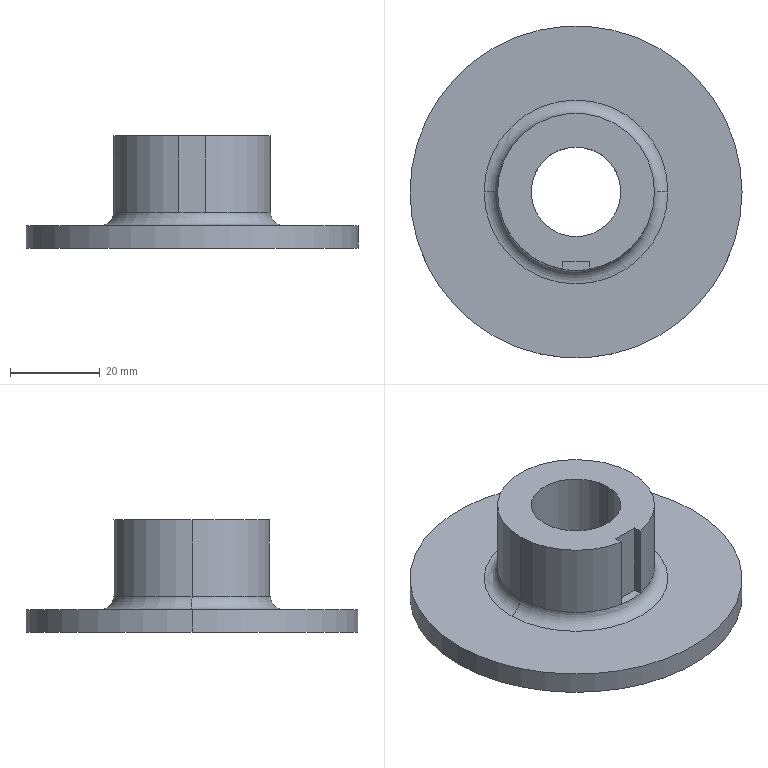Part | SolidWorks | features ICE 3, Extrusion 1, Fillet 1 | 1 solid | 16 faces | box 74 x 74 x 25 mm | volume 32918 mm3 | cylinder 7 | plane 7 | torus 2 | commonest cylinder face diameters 35 x3 20 x2 74 x2
STEP:
#1=CARTESIAN_POINT('',(-17.5,0.,8.));
#2=VERTEX_POINT('',#1);
#3=CARTESIAN_POINT('',(-3.,-17.241,8.));
#4=VERTEX_POINT('',#3);
#5=CARTESIAN_POINT('',(0.,0.,8.));
#6=DIRECTION('',(0.,0.,1.));
#7=DIRECTION('',(1.,0.,0.));
#8=AXIS2_PLACEMENT_3D('',#5,#6,#7);
#9=CIRCLE('',#8,17.5);
#10=EDGE_CURVE('',#2,#4,#9,.T.);
#11=ORIENTED_EDGE('',*,*,#10,.F.);
#12=CARTESIAN_POINT('',(-20.5,0.,5.));
#13=VERTEX_POINT('',#12);
#14=CARTESIAN_POINT('',(-20.5,0.,8.));
#15=DIRECTION('',(0.,1.,0.));
#16=DIRECTION('',(-1.,0.,0.));
#17=AXIS2_PLACEMENT_3D('',#14,#15,#16);
#18=CIRCLE('',#17,3.);
#19=EDGE_CURVE('',#2,#13,#18,.T.);
#20=ORIENTED_EDGE('',*,*,#19,.T.);
#21=CARTESIAN_POINT('',(20.5,0.,5.));
#22=VERTEX_POINT('',#21);
#23=CARTESIAN_POINT('',(0.,0.,5.));
#24=DIRECTION('',(0.,0.,-1.));
#25=DIRECTION('',(1.,0.,0.));
#26=AXIS2_PLACEMENT_3D('',#23,#24,#25);
#27=CIRCLE('',#26,20.5);
#28=EDGE_CURVE('',#22,#13,#27,.T.);
#29=ORIENTED_EDGE('',*,*,#28,.F.);
#30=CARTESIAN_POINT('',(17.5,0.,8.));
#31=VERTEX_POINT('',#30);
#32=CARTESIAN_POINT('',(20.5,0.,8.));
#33=DIRECTION('',(0.,-1.,0.));
#34=DIRECTION('',(0.,0.,-1.));
#35=AXIS2_PLACEMENT_3D('',#32,#33,#34);
#36=CIRCLE('',#35,3.);
#37=EDGE_CURVE('',#31,#22,#36,.T.);
#38=ORIENTED_EDGE('',*,*,#37,.F.);
#39=CARTESIAN_POINT('',(3.,-17.241,8.));
#40=VERTEX_POINT('',#39);
#41=CARTESIAN_POINT('',(0.,0.,8.));
#42=DIRECTION('',(0.,0.,1.));
#43=DIRECTION('',(1.,0.,0.));
#44=AXIS2_PLACEMENT_3D('',#41,#42,#43);
#45=CIRCLE('',#44,17.5);
#46=EDGE_CURVE('',#40,#31,#45,.T.);
#47=ORIENTED_EDGE('',*,*,#46,.F.);
#48=CARTESIAN_POINT('',(0.,0.,8.));
#49=DIRECTION('',(0.,0.,1.));
#50=DIRECTION('',(1.,0.,0.));
#51=AXIS2_PLACEMENT_3D('',#48,#49,#50);
#52=CIRCLE('',#51,17.5);
#53=EDGE_CURVE('',#4,#40,#52,.T.);
#54=ORIENTED_EDGE('',*,*,#53,.F.);
#55=EDGE_LOOP('',(#11,#20,#29,#38,#47,#54));
#56=FACE_OUTER_BOUND('',#55,.T.);
#57=CARTESIAN_POINT('',(0.,0.,8.));
#58=DIRECTION('',(0.,0.,1.));
#59=DIRECTION('',(1.,0.,0.));
#60=AXIS2_PLACEMENT_3D('',#57,#58,#59);
#61=TOROIDAL_SURFACE('',#60,20.5,3.);
#62=ADVANCED_FACE('',(#56),#61,.F.);
#63=CARTESIAN_POINT('',(-10.,0.,25.));
#64=VERTEX_POINT('',#63);
#65=CARTESIAN_POINT('',(10.,0.,25.));
#66=VERTEX_POINT('',#65);
#67=CARTESIAN_POINT('',(0.,0.,25.));
#68=DIRECTION('',(0.,0.,1.));
#69=DIRECTION('',(1.,0.,0.));
#70=AXIS2_PLACEMENT_3D('',#67,#68,#69);
#71=CIRCLE('',#70,10.);
#72=EDGE_CURVE('',#64,#66,#71,.T.);
#73=ORIENTED_EDGE('',*,*,#72,.T.);
#74=CARTESIAN_POINT('',(10.,0.,0.));
#75=VERTEX_POINT('',#74);
#76=CARTESIAN_POINT('',(10.,0.,25.));
#77=DIRECTION('',(0.,0.,-1.));
#78=VECTOR('',#77,1000.);
#79=LINE('',#76,#78);
#80=EDGE_CURVE('',#66,#75,#79,.T.);
#81=ORIENTED_EDGE('',*,*,#80,.T.);
#82=CARTESIAN_POINT('',(-10.,0.,0.));
#83=VERTEX_POINT('',#82);
#84=CARTESIAN_POINT('',(0.,0.,0.));
#85=DIRECTION('',(0.,0.,1.));
#86=DIRECTION('',(1.,0.,0.));
#87=AXIS2_PLACEMENT_3D('',#84,#85,#86);
#88=CIRCLE('',#87,10.);
#89=EDGE_CURVE('',#83,#75,#88,.T.);
#90=ORIENTED_EDGE('',*,*,#89,.F.);
#91=CARTESIAN_POINT('',(-10.,0.,25.));
#92=DIRECTION('',(0.,0.,-1.));
#93=VECTOR('',#92,1000.);
#94=LINE('',#91,#93);
#95=EDGE_CURVE('',#64,#83,#94,.T.);
#96=ORIENTED_EDGE('',*,*,#95,.F.);
#97=EDGE_LOOP('',(#73,#81,#90,#96));
#98=FACE_OUTER_BOUND('',#97,.T.);
#99=CARTESIAN_POINT('',(0.,0.,25.));
#100=DIRECTION('',(0.,0.,-1.));
#101=DIRECTION('',(-1.,0.,0.));
#102=AXIS2_PLACEMENT_3D('',#99,#100,#101);
#103=CYLINDRICAL_SURFACE('',#102,10.);
#104=ADVANCED_FACE('',(#98),#103,.F.);
#105=CARTESIAN_POINT('',(17.5,0.,25.));
#106=VERTEX_POINT('',#105);
#107=CARTESIAN_POINT('',(-17.5,0.,25.));
#108=VERTEX_POINT('',#107);
#109=CARTESIAN_POINT('',(0.,0.,25.));
#110=DIRECTION('',(0.,0.,1.));
#111=DIRECTION('',(1.,0.,0.));
#112=AXIS2_PLACEMENT_3D('',#109,#110,#111);
#113=CIRCLE('',#112,17.5);
#114=EDGE_CURVE('',#106,#108,#113,.T.);
#115=ORIENTED_EDGE('',*,*,#114,.F.);
#116=CARTESIAN_POINT('',(17.5,0.,25.));
#117=DIRECTION('',(0.,0.,-1.));
#118=VECTOR('',#117,1000.);
#119=LINE('',#116,#118);
#120=EDGE_CURVE('',#106,#31,#119,.T.);
#121=ORIENTED_EDGE('',*,*,#120,.T.);
#122=CARTESIAN_POINT('',(0.,0.,8.));
#123=DIRECTION('',(0.,0.,1.));
#124=DIRECTION('',(1.,0.,0.));
#125=AXIS2_PLACEMENT_3D('',#122,#123,#124);
#126=CIRCLE('',#125,17.5);
#127=EDGE_CURVE('',#31,#2,#126,.T.);
#128=ORIENTED_EDGE('',*,*,#127,.T.);
#129=CARTESIAN_POINT('',(-17.5,0.,25.));
#130=DIRECTION('',(0.,0.,-1.));
#131=VECTOR('',#130,1000.);
#132=LINE('',#129,#131);
#133=EDGE_CURVE('',#108,#2,#132,.T.);
#134=ORIENTED_EDGE('',*,*,#133,.F.);
#135=EDGE_LOOP('',(#115,#121,#128,#134));
#136=FACE_OUTER_BOUND('',#135,.T.);
#137=CARTESIAN_POINT('',(0.,0.,25.));
#138=DIRECTION('',(0.,0.,-1.));
#139=DIRECTION('',(-1.,0.,0.));
#140=AXIS2_PLACEMENT_3D('',#137,#138,#139);
#141=CYLINDRICAL_SURFACE('',#140,17.5);
#142=ADVANCED_FACE('',(#136),#141,.T.);
#143=CARTESIAN_POINT('',(-3.,-17.241,25.));
#144=VERTEX_POINT('',#143);
#145=CARTESIAN_POINT('',(0.,0.,25.));
#146=DIRECTION('',(0.,0.,1.));
#147=DIRECTION('',(1.,0.,0.));
#148=AXIS2_PLACEMENT_3D('',#145,#146,#147);
#149=CIRCLE('',#148,17.5);
#150=EDGE_CURVE('',#108,#144,#149,.T.);
#151=ORIENTED_EDGE('',*,*,#150,.F.);
#152=ORIENTED_EDGE('',*,*,#133,.T.);
#153=ORIENTED_EDGE('',*,*,#10,.T.);
#154=CARTESIAN_POINT('',(-3.,-17.241,25.));
#155=DIRECTION('',(0.,0.,1.));
#156=VECTOR('',#155,1000.);
#157=LINE('',#154,#156);
#158=EDGE_CURVE('',#4,#144,#157,.T.);
#159=ORIENTED_EDGE('',*,*,#158,.T.);
#160=EDGE_LOOP('',(#151,#152,#153,#159));
#161=FACE_OUTER_BOUND('',#160,.T.);
#162=CARTESIAN_POINT('',(0.,0.,25.));
#163=DIRECTION('',(0.,0.,-1.));
#164=DIRECTION('',(-1.,0.,0.));
#165=AXIS2_PLACEMENT_3D('',#162,#163,#164);
#166=CYLINDRICAL_SURFACE('',#165,17.5);
#167=ADVANCED_FACE('',(#161),#166,.T.);
#168=CARTESIAN_POINT('',(37.,0.,5.));
#169=VERTEX_POINT('',#168);
#170=CARTESIAN_POINT('',(-37.,0.,5.));
#171=VERTEX_POINT('',#170);
#172=CARTESIAN_POINT('',(0.,0.,5.));
#173=DIRECTION('',(0.,0.,1.));
#174=DIRECTION('',(1.,0.,0.));
#175=AXIS2_PLACEMENT_3D('',#172,#173,#174);
#176=CIRCLE('',#175,37.);
#177=EDGE_CURVE('',#169,#171,#176,.T.);
#178=ORIENTED_EDGE('',*,*,#177,.F.);
#179=CARTESIAN_POINT('',(37.,0.,0.));
#180=VERTEX_POINT('',#179);
#181=CARTESIAN_POINT('',(37.,0.,5.));
#182=DIRECTION('',(0.,0.,-1.));
#183=VECTOR('',#182,1000.);
#184=LINE('',#181,#183);
#185=EDGE_CURVE('',#169,#180,#184,.T.);
#186=ORIENTED_EDGE('',*,*,#185,.T.);
#187=CARTESIAN_POINT('',(-37.,0.,0.));
#188=VERTEX_POINT('',#187);
#189=CARTESIAN_POINT('',(0.,0.,0.));
#190=DIRECTION('',(0.,0.,1.));
#191=DIRECTION('',(1.,0.,0.));
#192=AXIS2_PLACEMENT_3D('',#189,#190,#191);
#193=CIRCLE('',#192,37.);
#194=EDGE_CURVE('',#180,#188,#193,.T.);
#195=ORIENTED_EDGE('',*,*,#194,.T.);
#196=CARTESIAN_POINT('',(-37.,0.,5.));
#197=DIRECTION('',(0.,0.,-1.));
#198=VECTOR('',#197,1000.);
#199=LINE('',#196,#198);
#200=EDGE_CURVE('',#171,#188,#199,.T.);
#201=ORIENTED_EDGE('',*,*,#200,.F.);
#202=EDGE_LOOP('',(#178,#186,#195,#201));
#203=FACE_OUTER_BOUND('',#202,.T.);
#204=CARTESIAN_POINT('',(0.,0.,5.));
#205=DIRECTION('',(0.,0.,-1.));
#206=DIRECTION('',(-1.,0.,0.));
#207=AXIS2_PLACEMENT_3D('',#204,#205,#206);
#208=CYLINDRICAL_SURFACE('',#207,37.);
#209=ADVANCED_FACE('',(#203),#208,.T.);
#210=ORIENTED_EDGE('',*,*,#28,.T.);
#211=CARTESIAN_POINT('',(0.,0.,5.));
#212=DIRECTION('',(0.,0.,-1.));
#213=DIRECTION('',(1.,0.,0.));
#214=AXIS2_PLACEMENT_3D('',#211,#212,#213);
#215=CIRCLE('',#214,20.5);
#216=EDGE_CURVE('',#13,#22,#215,.T.);
#217=ORIENTED_EDGE('',*,*,#216,.T.);
#218=EDGE_LOOP('',(#210,#217));
#219=FACE_BOUND('',#218,.T.);
#220=CARTESIAN_POINT('',(0.,0.,5.));
#221=DIRECTION('',(0.,0.,1.));
#222=DIRECTION('',(1.,0.,0.));
#223=AXIS2_PLACEMENT_3D('',#220,#221,#222);
#224=CIRCLE('',#223,37.);
#225=EDGE_CURVE('',#171,#169,#224,.T.);
#226=ORIENTED_EDGE('',*,*,#225,.T.);
#227=ORIENTED_EDGE('',*,*,#177,.T.);
#228=EDGE_LOOP('',(#226,#227));
#229=FACE_OUTER_BOUND('',#228,.T.);
#230=CARTESIAN_POINT('',(0.,0.,5.));
#231=DIRECTION('',(0.,0.,1.));
#232=DIRECTION('',(1.,0.,0.));
#233=AXIS2_PLACEMENT_3D('',#230,#231,#232);
#234=PLANE('',#233);
#235=ADVANCED_FACE('',(#219,#229),#234,.T.);
#236=ORIENTED_EDGE('',*,*,#185,.F.);
#237=ORIENTED_EDGE('',*,*,#225,.F.);
#238=ORIENTED_EDGE('',*,*,#200,.T.);
#239=CARTESIAN_POINT('',(0.,0.,0.));
#240=DIRECTION('',(0.,0.,1.));
#241=DIRECTION('',(1.,0.,0.));
#242=AXIS2_PLACEMENT_3D('',#239,#240,#241);
#243=CIRCLE('',#242,37.);
#244=EDGE_CURVE('',#188,#180,#243,.T.);
#245=ORIENTED_EDGE('',*,*,#244,.T.);
#246=EDGE_LOOP('',(#236,#237,#238,#245));
#247=FACE_OUTER_BOUND('',#246,.T.);
#248=CARTESIAN_POINT('',(0.,0.,5.));
#249=DIRECTION('',(0.,0.,-1.));
#250=DIRECTION('',(-1.,0.,0.));
#251=AXIS2_PLACEMENT_3D('',#248,#249,#250);
#252=CYLINDRICAL_SURFACE('',#251,37.);
#253=ADVANCED_FACE('',(#247),#252,.T.);
#254=ORIENTED_EDGE('',*,*,#89,.T.);
#255=CARTESIAN_POINT('',(0.,0.,0.));
#256=DIRECTION('',(0.,0.,1.));
#257=DIRECTION('',(1.,0.,0.));
#258=AXIS2_PLACEMENT_3D('',#255,#256,#257);
#259=CIRCLE('',#258,10.);
#260=EDGE_CURVE('',#75,#83,#259,.T.);
#261=ORIENTED_EDGE('',*,*,#260,.T.);
#262=EDGE_LOOP('',(#254,#261));
#263=FACE_BOUND('',#262,.T.);
#264=ORIENTED_EDGE('',*,*,#244,.F.);
#265=ORIENTED_EDGE('',*,*,#194,.F.);
#266=EDGE_LOOP('',(#264,#265));
#267=FACE_OUTER_BOUND('',#266,.T.);
#268=CARTESIAN_POINT('',(0.,0.,0.));
#269=DIRECTION('',(0.,0.,1.));
#270=DIRECTION('',(1.,0.,0.));
#271=AXIS2_PLACEMENT_3D('',#268,#269,#270);
#272=PLANE('',#271);
#273=ADVANCED_FACE('',(#263,#267),#272,.F.);
#274=CARTESIAN_POINT('',(3.,-17.241,25.));
#275=VERTEX_POINT('',#274);
#276=CARTESIAN_POINT('',(3.,-15.5,25.));
#277=VERTEX_POINT('',#276);
#278=CARTESIAN_POINT('',(3.,-19.5,25.));
#279=DIRECTION('',(0.,1.,0.));
#280=VECTOR('',#279,1000.);
#281=LINE('',#278,#280);
#282=EDGE_CURVE('',#275,#277,#281,.T.);
#283=ORIENTED_EDGE('',*,*,#282,.F.);
#284=CARTESIAN_POINT('',(0.,0.,25.));
#285=DIRECTION('',(0.,0.,1.));
#286=DIRECTION('',(1.,0.,0.));
#287=AXIS2_PLACEMENT_3D('',#284,#285,#286);
#288=CIRCLE('',#287,17.5);
#289=EDGE_CURVE('',#275,#106,#288,.T.);
#290=ORIENTED_EDGE('',*,*,#289,.T.);
#291=ORIENTED_EDGE('',*,*,#114,.T.);
#292=ORIENTED_EDGE('',*,*,#150,.T.);
#293=CARTESIAN_POINT('',(-3.,-15.5,25.));
#294=VERTEX_POINT('',#293);
#295=CARTESIAN_POINT('',(-3.,-19.5,25.));
#296=DIRECTION('',(0.,-1.,0.));
#297=VECTOR('',#296,1000.);
#298=LINE('',#295,#297);
#299=EDGE_CURVE('',#294,#144,#298,.T.);
#300=ORIENTED_EDGE('',*,*,#299,.F.);
#301=CARTESIAN_POINT('',(-3.,-15.5,25.));
#302=DIRECTION('',(-1.,0.,0.));
#303=VECTOR('',#302,1000.);
#304=LINE('',#301,#303);
#305=EDGE_CURVE('',#277,#294,#304,.T.);
#306=ORIENTED_EDGE('',*,*,#305,.F.);
#307=EDGE_LOOP('',(#283,#290,#291,#292,#300,#306));
#308=FACE_OUTER_BOUND('',#307,.T.);
#309=ORIENTED_EDGE('',*,*,#72,.F.);
#310=CARTESIAN_POINT('',(0.,0.,25.));
#311=DIRECTION('',(0.,0.,1.));
#312=DIRECTION('',(1.,0.,0.));
#313=AXIS2_PLACEMENT_3D('',#310,#311,#312);
#314=CIRCLE('',#313,10.);
#315=EDGE_CURVE('',#66,#64,#314,.T.);
#316=ORIENTED_EDGE('',*,*,#315,.F.);
#317=EDGE_LOOP('',(#309,#316));
#318=FACE_BOUND('',#317,.T.);
#319=CARTESIAN_POINT('',(0.,0.,25.));
#320=DIRECTION('',(0.,0.,1.));
#321=DIRECTION('',(1.,0.,0.));
#322=AXIS2_PLACEMENT_3D('',#319,#320,#321);
#323=PLANE('',#322);
#324=ADVANCED_FACE('',(#308,#318),#323,.T.);
#325=ORIENTED_EDGE('',*,*,#120,.F.);
#326=ORIENTED_EDGE('',*,*,#289,.F.);
#327=CARTESIAN_POINT('',(3.,-17.241,25.));
#328=DIRECTION('',(0.,0.,-1.));
#329=VECTOR('',#328,1000.);
#330=LINE('',#327,#329);
#331=EDGE_CURVE('',#275,#40,#330,.T.);
#332=ORIENTED_EDGE('',*,*,#331,.T.);
#333=ORIENTED_EDGE('',*,*,#46,.T.);
#334=EDGE_LOOP('',(#325,#326,#332,#333));
#335=FACE_OUTER_BOUND('',#334,.T.);
#336=CARTESIAN_POINT('',(0.,0.,25.));
#337=DIRECTION('',(0.,0.,-1.));
#338=DIRECTION('',(-1.,0.,0.));
#339=AXIS2_PLACEMENT_3D('',#336,#337,#338);
#340=CYLINDRICAL_SURFACE('',#339,17.5);
#341=ADVANCED_FACE('',(#335),#340,.T.);
#342=ORIENTED_EDGE('',*,*,#80,.F.);
#343=ORIENTED_EDGE('',*,*,#315,.T.);
#344=ORIENTED_EDGE('',*,*,#95,.T.);
#345=ORIENTED_EDGE('',*,*,#260,.F.);
#346=EDGE_LOOP('',(#342,#343,#344,#345));
#347=FACE_OUTER_BOUND('',#346,.T.);
#348=CARTESIAN_POINT('',(0.,0.,25.));
#349=DIRECTION('',(0.,0.,-1.));
#350=DIRECTION('',(-1.,0.,0.));
#351=AXIS2_PLACEMENT_3D('',#348,#349,#350);
#352=CYLINDRICAL_SURFACE('',#351,10.);
#353=ADVANCED_FACE('',(#347),#352,.F.);
#354=ORIENTED_EDGE('',*,*,#19,.F.);
#355=ORIENTED_EDGE('',*,*,#127,.F.);
#356=ORIENTED_EDGE('',*,*,#37,.T.);
#357=ORIENTED_EDGE('',*,*,#216,.F.);
#358=EDGE_LOOP('',(#354,#355,#356,#357));
#359=FACE_OUTER_BOUND('',#358,.T.);
#360=CARTESIAN_POINT('',(0.,0.,8.));
#361=DIRECTION('',(0.,0.,1.));
#362=DIRECTION('',(1.,0.,0.));
#363=AXIS2_PLACEMENT_3D('',#360,#361,#362);
#364=TOROIDAL_SURFACE('',#363,20.5,3.);
#365=ADVANCED_FACE('',(#359),#364,.F.);
#366=ORIENTED_EDGE('',*,*,#282,.T.);
#367=CARTESIAN_POINT('',(3.,-15.5,8.));
#368=VERTEX_POINT('',#367);
#369=CARTESIAN_POINT('',(3.,-15.5,-2.211));
#370=DIRECTION('',(0.,0.,1.));
#371=VECTOR('',#370,1000.);
#372=LINE('',#369,#371);
#373=EDGE_CURVE('',#368,#277,#372,.T.);
#374=ORIENTED_EDGE('',*,*,#373,.F.);
#375=CARTESIAN_POINT('',(3.,-19.5,8.));
#376=DIRECTION('',(0.,-1.,0.));
#377=VECTOR('',#376,1000.);
#378=LINE('',#375,#377);
#379=EDGE_CURVE('',#368,#40,#378,.T.);
#380=ORIENTED_EDGE('',*,*,#379,.T.);
#381=ORIENTED_EDGE('',*,*,#331,.F.);
#382=EDGE_LOOP('',(#366,#374,#380,#381));
#383=FACE_OUTER_BOUND('',#382,.T.);
#384=CARTESIAN_POINT('',(3.,-19.5,-2.211));
#385=DIRECTION('',(1.,0.,0.));
#386=DIRECTION('',(0.,0.,-1.));
#387=AXIS2_PLACEMENT_3D('',#384,#385,#386);
#388=PLANE('',#387);
#389=ADVANCED_FACE('',(#383),#388,.F.);
#390=CARTESIAN_POINT('',(-3.,-15.5,8.));
#391=VERTEX_POINT('',#390);
#392=CARTESIAN_POINT('',(-3.,-19.5,8.));
#393=DIRECTION('',(0.,1.,0.));
#394=VECTOR('',#393,1000.);
#395=LINE('',#392,#394);
#396=EDGE_CURVE('',#4,#391,#395,.T.);
#397=ORIENTED_EDGE('',*,*,#396,.T.);
#398=CARTESIAN_POINT('',(-3.,-15.5,-2.211));
#399=DIRECTION('',(0.,0.,1.));
#400=VECTOR('',#399,1000.);
#401=LINE('',#398,#400);
#402=EDGE_CURVE('',#391,#294,#401,.T.);
#403=ORIENTED_EDGE('',*,*,#402,.T.);
#404=ORIENTED_EDGE('',*,*,#299,.T.);
#405=ORIENTED_EDGE('',*,*,#158,.F.);
#406=EDGE_LOOP('',(#397,#403,#404,#405));
#407=FACE_OUTER_BOUND('',#406,.T.);
#408=CARTESIAN_POINT('',(-3.,-19.5,-2.211));
#409=DIRECTION('',(-1.,0.,0.));
#410=DIRECTION('',(0.,0.,1.));
#411=AXIS2_PLACEMENT_3D('',#408,#409,#410);
#412=PLANE('',#411);
#413=ADVANCED_FACE('',(#407),#412,.F.);
#414=ORIENTED_EDGE('',*,*,#53,.T.);
#415=ORIENTED_EDGE('',*,*,#379,.F.);
#416=CARTESIAN_POINT('',(-3.,-15.5,8.));
#417=DIRECTION('',(1.,0.,0.));
#418=VECTOR('',#417,1000.);
#419=LINE('',#416,#418);
#420=EDGE_CURVE('',#391,#368,#419,.T.);
#421=ORIENTED_EDGE('',*,*,#420,.F.);
#422=ORIENTED_EDGE('',*,*,#396,.F.);
#423=EDGE_LOOP('',(#414,#415,#421,#422));
#424=FACE_OUTER_BOUND('',#423,.T.);
#425=CARTESIAN_POINT('',(0.,0.,8.));
#426=DIRECTION('',(0.,0.,1.));
#427=DIRECTION('',(1.,0.,0.));
#428=AXIS2_PLACEMENT_3D('',#425,#426,#427);
#429=PLANE('',#428);
#430=ADVANCED_FACE('',(#424),#429,.T.);
#431=ORIENTED_EDGE('',*,*,#420,.T.);
#432=ORIENTED_EDGE('',*,*,#373,.T.);
#433=ORIENTED_EDGE('',*,*,#305,.T.);
#434=ORIENTED_EDGE('',*,*,#402,.F.);
#435=EDGE_LOOP('',(#431,#432,#433,#434));
#436=FACE_OUTER_BOUND('',#435,.T.);
#437=CARTESIAN_POINT('',(-3.,-15.5,-2.211));
#438=DIRECTION('',(0.,1.,0.));
#439=DIRECTION('',(0.,0.,1.));
#440=AXIS2_PLACEMENT_3D('',#437,#438,#439);
#441=PLANE('',#440);
#442=ADVANCED_FACE('',(#436),#441,.F.);
#443=CLOSED_SHELL('',(#62,#104,#142,#167,#209,#235,#253,#273,#324,#341,#353,#365,#389,#413,#430,#442));
#444=MANIFOLD_SOLID_BREP('',#443);
#445=CARTESIAN_POINT('',(0.,0.,0.));
#446=DIRECTION('',(0.,0.,1.));
#447=DIRECTION('',(1.,0.,0.));
#448=AXIS2_PLACEMENT_3D('',#445,#446,#447);
#449=(LENGTH_UNIT()NAMED_UNIT(*)SI_UNIT(.MILLI.,.METRE.));
#450=UNCERTAINTY_MEASURE_WITH_UNIT(LENGTH_MEASURE(0.00001),#449,'','');
#451=(NAMED_UNIT(*)PLANE_ANGLE_UNIT()SI_UNIT($,.RADIAN.));
#452=(NAMED_UNIT(*)SI_UNIT($,.STERADIAN.)SOLID_ANGLE_UNIT());
#453=(GEOMETRIC_REPRESENTATION_CONTEXT(3)GLOBAL_UNCERTAINTY_ASSIGNED_CONTEXT((#450))GLOBAL_UNIT_ASSIGNED_CONTEXT((#449,#451,#452))REPRESENTATION_CONTEXT('',''));
#454=ADVANCED_BREP_SHAPE_REPRESENTATION('',(#444,#448),#453);